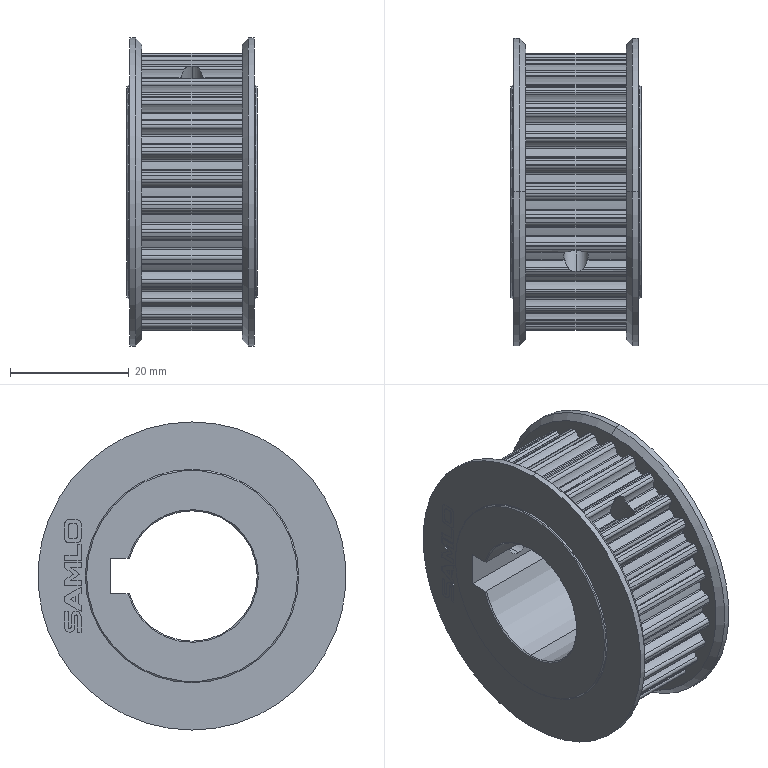Part | SolidWorks | features BaseBody 1 | 1 solid | 379 faces | box 22 x 52 x 52 mm | volume 27109 mm3 | cylinder 305 | plane 61 | cone 13 | commonest cylinder face diameters 1.1 x73 0.5 x72 6.55 x68 43.25 x32 46.79 x31 0.643 x4